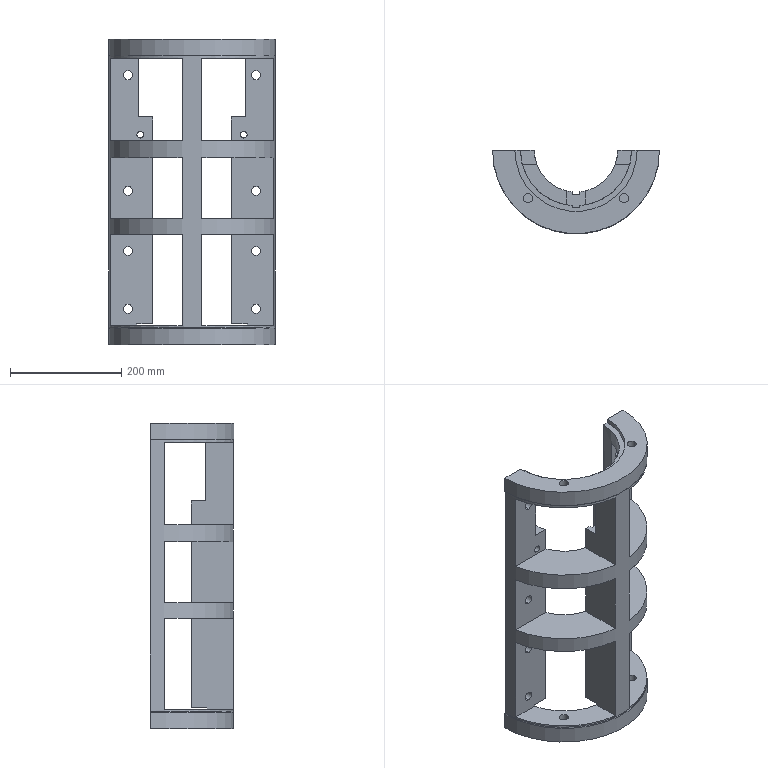Part | SolidWorks | features ICE 19, HoleWzd 4, RevCut 4, BaseBody 1 | 1 solid | 88 faces | box 300 x 150 x 550 mm | volume 5063192 mm3 | plane 47 | cylinder 40 | torus 1 | commonest cylinder face diameters 16 x16 16.5 x8 12 x4 20.5 x2 150 x2 200 x2